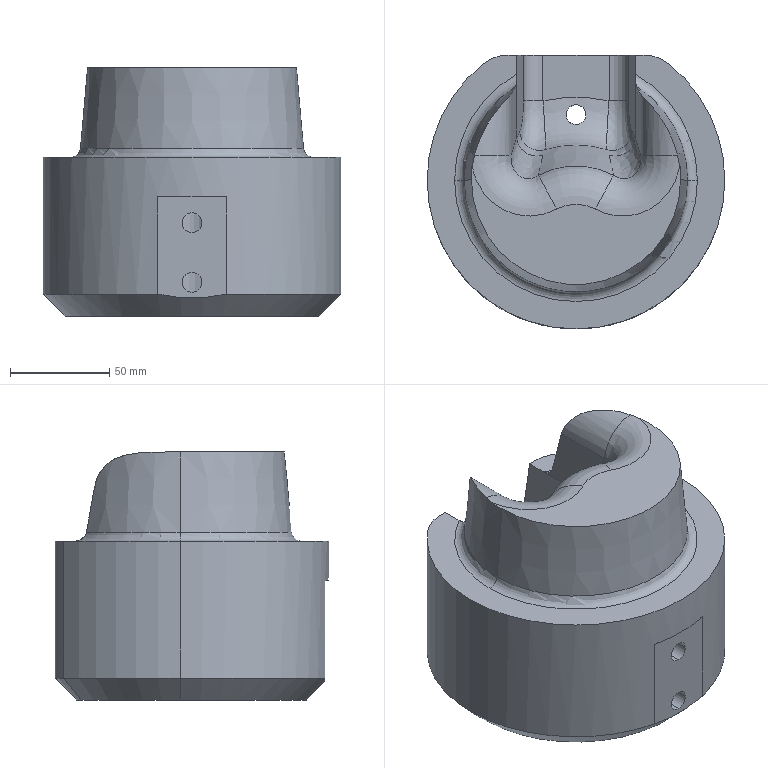Part | SolidWorks | features BaseBody 1 | 1 solid | 67 faces | box 150 x 138 x 125 mm | volume 1503257 mm3 | cylinder 25 | cone 15 | plane 14 | spline 8 | torus 5 | commonest cylinder face diameters 10 x6 10.5 x4 20 x4 40 x4 150 x3 11 x2